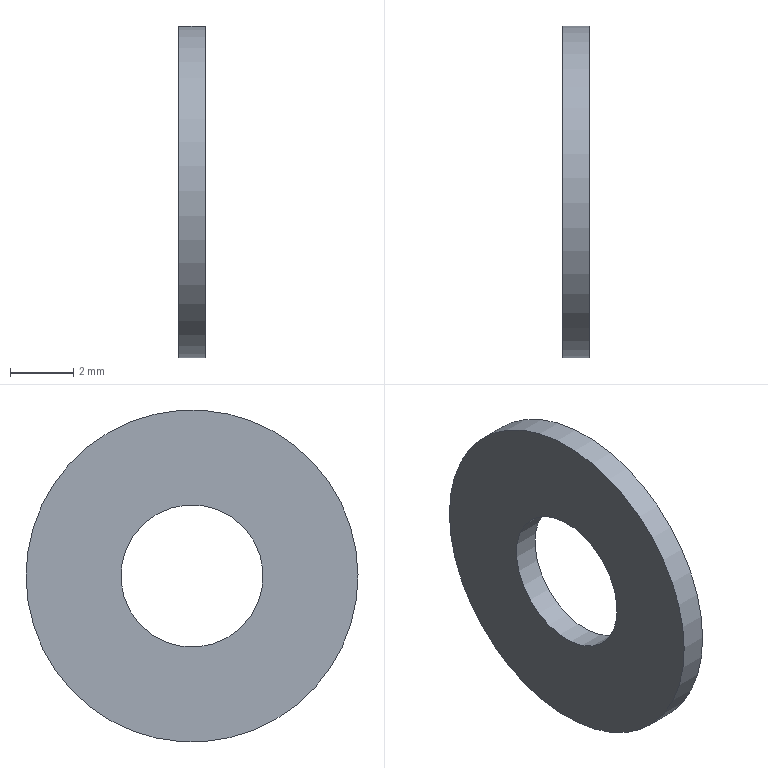Part | NX | features TAM02-M3-L8-003 2 | 1 solid | 4 faces | box 0.825 x 10.5 x 10.5 mm | volume 58.316 mm3 | cylinder 2 | plane 2 | commonest cylinder face diameters 4.5 x1 10.5 x1
STEP:
#1=CARTESIAN_POINT('',(132.123,-46.525,-32.904));
#2=VERTEX_POINT('',#1);
#3=CARTESIAN_POINT('',(132.123,-42.7,-36.5));
#4=DIRECTION('',(-1.,0.,0.));
#5=DIRECTION('',(0.,-0.7285,0.685));
#6=AXIS2_PLACEMENT_3D('',#3,#4,#5);
#7=CIRCLE('',#6,5.25);
#8=EDGE_CURVE('',#2,#2,#7,.T.);
#9=ORIENTED_EDGE('',*,*,#8,.T.);
#10=EDGE_LOOP('',(#9));
#11=FACE_BOUND('',#10,.T.);
#12=CARTESIAN_POINT('',(131.298,-46.525,-32.904));
#13=VERTEX_POINT('',#12);
#14=CARTESIAN_POINT('',(131.298,-42.7,-36.5));
#15=DIRECTION('',(-1.,0.,0.));
#16=DIRECTION('',(0.,-0.7285,0.685));
#17=AXIS2_PLACEMENT_3D('',#14,#15,#16);
#18=CIRCLE('',#17,5.25);
#19=EDGE_CURVE('',#13,#13,#18,.T.);
#20=ORIENTED_EDGE('',*,*,#19,.F.);
#21=EDGE_LOOP('',(#20));
#22=FACE_BOUND('',#21,.T.);
#23=CARTESIAN_POINT('',(131.298,-42.7,-36.5));
#24=DIRECTION('',(1.,0.,0.));
#25=DIRECTION('',(0.,0.7285,-0.685));
#26=AXIS2_PLACEMENT_3D('',#23,#24,#25);
#27=CYLINDRICAL_SURFACE('',#26,5.25);
#28=ADVANCED_FACE('',(#11,#22),#27,.T.);
#29=CARTESIAN_POINT('',(132.123,-44.339,-34.959));
#30=VERTEX_POINT('',#29);
#31=CARTESIAN_POINT('',(132.123,-42.7,-36.5));
#32=DIRECTION('',(-1.,0.,0.));
#33=DIRECTION('',(0.,-0.7285,0.685));
#34=AXIS2_PLACEMENT_3D('',#31,#32,#33);
#35=CIRCLE('',#34,2.25);
#36=EDGE_CURVE('',#30,#30,#35,.T.);
#37=ORIENTED_EDGE('',*,*,#36,.F.);
#38=EDGE_LOOP('',(#37));
#39=FACE_BOUND('',#38,.T.);
#40=CARTESIAN_POINT('',(131.298,-44.339,-34.959));
#41=VERTEX_POINT('',#40);
#42=CARTESIAN_POINT('',(131.298,-42.7,-36.5));
#43=DIRECTION('',(-1.,0.,0.));
#44=DIRECTION('',(0.,-0.7285,0.685));
#45=AXIS2_PLACEMENT_3D('',#42,#43,#44);
#46=CIRCLE('',#45,2.25);
#47=EDGE_CURVE('',#41,#41,#46,.T.);
#48=ORIENTED_EDGE('',*,*,#47,.T.);
#49=EDGE_LOOP('',(#48));
#50=FACE_BOUND('',#49,.T.);
#51=CARTESIAN_POINT('',(131.298,-42.7,-36.5));
#52=DIRECTION('',(1.,0.,0.));
#53=DIRECTION('',(0.,0.7285,-0.685));
#54=AXIS2_PLACEMENT_3D('',#51,#52,#53);
#55=CYLINDRICAL_SURFACE('',#54,2.25);
#56=ADVANCED_FACE('',(#39,#50),#55,.F.);
#57=ORIENTED_EDGE('',*,*,#47,.F.);
#58=EDGE_LOOP('',(#57));
#59=FACE_BOUND('',#58,.T.);
#60=ORIENTED_EDGE('',*,*,#19,.T.);
#61=EDGE_LOOP('',(#60));
#62=FACE_BOUND('',#61,.T.);
#63=CARTESIAN_POINT('',(131.298,-42.7,-36.5));
#64=DIRECTION('',(-1.,0.,0.));
#65=DIRECTION('',(0.,-0.7285,0.685));
#66=AXIS2_PLACEMENT_3D('',#63,#64,#65);
#67=PLANE('',#66);
#68=ADVANCED_FACE('',(#59,#62),#67,.T.);
#69=ORIENTED_EDGE('',*,*,#36,.T.);
#70=EDGE_LOOP('',(#69));
#71=FACE_BOUND('',#70,.T.);
#72=ORIENTED_EDGE('',*,*,#8,.F.);
#73=EDGE_LOOP('',(#72));
#74=FACE_BOUND('',#73,.T.);
#75=CARTESIAN_POINT('',(132.123,-42.7,-36.5));
#76=DIRECTION('',(-1.,0.,0.));
#77=DIRECTION('',(0.,-0.7285,0.685));
#78=AXIS2_PLACEMENT_3D('',#75,#76,#77);
#79=PLANE('',#78);
#80=ADVANCED_FACE('',(#71,#74),#79,.F.);
#81=CLOSED_SHELL('',(#28,#56,#68,#80));
#82=MANIFOLD_SOLID_BREP('',#81);
#83=(LENGTH_UNIT()NAMED_UNIT(*)SI_UNIT(.MILLI.,.METRE.));
#84=UNCERTAINTY_MEASURE_WITH_UNIT(LENGTH_MEASURE(0.00001),#83,'','');
#85=(NAMED_UNIT(*)PLANE_ANGLE_UNIT()SI_UNIT($,.RADIAN.));
#86=(NAMED_UNIT(*)SI_UNIT($,.STERADIAN.)SOLID_ANGLE_UNIT());
#87=(GEOMETRIC_REPRESENTATION_CONTEXT(3)GLOBAL_UNCERTAINTY_ASSIGNED_CONTEXT((#84))GLOBAL_UNIT_ASSIGNED_CONTEXT((#83,#85,#86))REPRESENTATION_CONTEXT('',''));
#88=ADVANCED_BREP_SHAPE_REPRESENTATION('',(#82),#87);